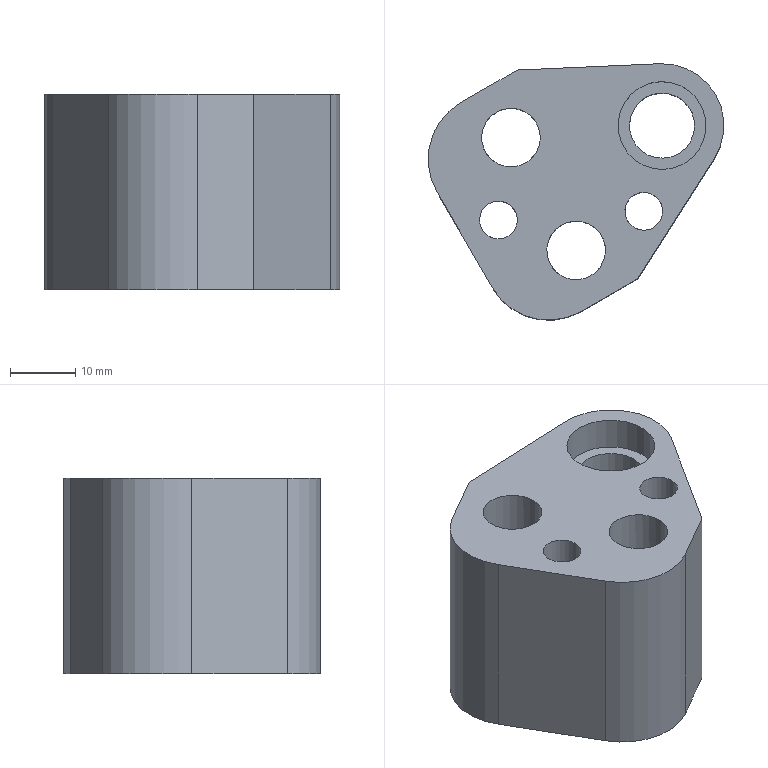Part | NX | features solid 2 | 1 solid | 25 faces | box 45.401 x 39.361 x 30 mm | volume 27576 mm3 | cylinder 13 | plane 12 | commonest cylinder face diameters 5.8 x2 8 x2 9 x2 14 x2 20 x2 10 x1
STEP:
#1=CARTESIAN_POINT('',(511.856,-185.624,74.));
#2=VERTEX_POINT('',#1);
#3=CARTESIAN_POINT('',(523.615,-167.196,74.));
#4=VERTEX_POINT('',#3);
#5=CARTESIAN_POINT('',(522.614,-168.764,74.));
#6=DIRECTION('',(0.5379,0.843,0.));
#7=VECTOR('',#6,1000.);
#8=LINE('',#5,#7);
#9=EDGE_CURVE('',#2,#4,#8,.T.);
#10=ORIENTED_EDGE('',*,*,#9,.T.);
#11=CARTESIAN_POINT('',(515.194,-152.611,74.));
#12=VERTEX_POINT('',#11);
#13=CARTESIAN_POINT('',(515.596,-162.103,74.));
#14=DIRECTION('',(0.,0.,-1.));
#15=DIRECTION('',(-0.5,0.866,0.));
#16=AXIS2_PLACEMENT_3D('',#13,#14,#15);
#17=CIRCLE('',#16,9.5);
#18=EDGE_CURVE('',#12,#4,#17,.T.);
#19=ORIENTED_EDGE('',*,*,#18,.F.);
#20=CARTESIAN_POINT('',(493.356,-153.581,74.));
#21=VERTEX_POINT('',#20);
#22=CARTESIAN_POINT('',(513.336,-152.694,74.));
#23=DIRECTION('',(-0.999,-0.04437,0.));
#24=VECTOR('',#23,1000.);
#25=LINE('',#22,#24);
#26=EDGE_CURVE('',#12,#21,#25,.T.);
#27=ORIENTED_EDGE('',*,*,#26,.T.);
#28=CARTESIAN_POINT('',(484.695,-158.581,74.));
#29=VERTEX_POINT('',#28);
#30=CARTESIAN_POINT('',(501.747,-148.736,74.));
#31=DIRECTION('',(0.866,0.5,0.));
#32=VECTOR('',#31,1000.);
#33=LINE('',#30,#32);
#34=EDGE_CURVE('',#29,#21,#33,.T.);
#35=ORIENTED_EDGE('',*,*,#34,.F.);
#36=CARTESIAN_POINT('',(481.035,-172.241,74.));
#37=VERTEX_POINT('',#36);
#38=CARTESIAN_POINT('',(489.695,-167.241,74.));
#39=DIRECTION('',(0.,0.,1.));
#40=DIRECTION('',(-0.5,-0.866,0.));
#41=AXIS2_PLACEMENT_3D('',#38,#39,#40);
#42=CIRCLE('',#41,10.);
#43=EDGE_CURVE('',#29,#37,#42,.T.);
#44=ORIENTED_EDGE('',*,*,#43,.T.);
#45=CARTESIAN_POINT('',(489.535,-186.964,74.));
#46=VERTEX_POINT('',#45);
#47=CARTESIAN_POINT('',(485.285,-179.603,74.));
#48=DIRECTION('',(-0.5,0.866,0.));
#49=VECTOR('',#48,1000.);
#50=LINE('',#47,#49);
#51=EDGE_CURVE('',#46,#37,#50,.T.);
#52=ORIENTED_EDGE('',*,*,#51,.F.);
#53=CARTESIAN_POINT('',(503.195,-190.624,74.));
#54=VERTEX_POINT('',#53);
#55=CARTESIAN_POINT('',(498.195,-181.964,74.));
#56=DIRECTION('',(0.,0.,1.));
#57=DIRECTION('',(-0.5,-0.866,0.));
#58=AXIS2_PLACEMENT_3D('',#55,#56,#57);
#59=CIRCLE('',#58,10.);
#60=EDGE_CURVE('',#46,#54,#59,.T.);
#61=ORIENTED_EDGE('',*,*,#60,.T.);
#62=CARTESIAN_POINT('',(520.247,-180.779,74.));
#63=DIRECTION('',(-0.866,-0.5,0.));
#64=VECTOR('',#63,1000.);
#65=LINE('',#62,#64);
#66=EDGE_CURVE('',#2,#54,#65,.T.);
#67=ORIENTED_EDGE('',*,*,#66,.F.);
#68=EDGE_LOOP('',(#10,#19,#27,#35,#44,#52,#61,#67));
#69=FACE_BOUND('',#68,.T.);
#70=CARTESIAN_POINT('',(489.031,-174.091,74.));
#71=VERTEX_POINT('',#70);
#72=CARTESIAN_POINT('',(490.481,-176.603,74.));
#73=DIRECTION('',(0.,0.,-1.));
#74=DIRECTION('',(-0.5,0.866,0.));
#75=AXIS2_PLACEMENT_3D('',#72,#73,#74);
#76=CIRCLE('',#75,2.9);
#77=EDGE_CURVE('',#71,#71,#76,.T.);
#78=ORIENTED_EDGE('',*,*,#77,.T.);
#79=EDGE_LOOP('',(#78));
#80=FACE_BOUND('',#79,.T.);
#81=CARTESIAN_POINT('',(511.352,-172.751,74.));
#82=VERTEX_POINT('',#81);
#83=CARTESIAN_POINT('',(512.802,-175.263,74.));
#84=DIRECTION('',(0.,0.,-1.));
#85=DIRECTION('',(-0.5,0.866,0.));
#86=AXIS2_PLACEMENT_3D('',#83,#84,#85);
#87=CIRCLE('',#86,2.9);
#88=EDGE_CURVE('',#82,#82,#87,.T.);
#89=ORIENTED_EDGE('',*,*,#88,.T.);
#90=EDGE_LOOP('',(#89));
#91=FACE_BOUND('',#90,.T.);
#92=CARTESIAN_POINT('',(500.159,-177.366,74.));
#93=VERTEX_POINT('',#92);
#94=CARTESIAN_POINT('',(502.409,-181.263,74.));
#95=DIRECTION('',(0.,0.,-1.));
#96=DIRECTION('',(-0.5,0.866,0.));
#97=AXIS2_PLACEMENT_3D('',#94,#95,#96);
#98=CIRCLE('',#97,4.5);
#99=EDGE_CURVE('',#93,#93,#98,.T.);
#100=ORIENTED_EDGE('',*,*,#99,.T.);
#101=EDGE_LOOP('',(#100));
#102=FACE_BOUND('',#101,.T.);
#103=CARTESIAN_POINT('',(490.159,-160.045,74.));
#104=VERTEX_POINT('',#103);
#105=CARTESIAN_POINT('',(492.409,-163.942,74.));
#106=DIRECTION('',(0.,0.,-1.));
#107=DIRECTION('',(-0.5,0.866,0.));
#108=AXIS2_PLACEMENT_3D('',#105,#106,#107);
#109=CIRCLE('',#108,4.5);
#110=EDGE_CURVE('',#104,#104,#109,.T.);
#111=ORIENTED_EDGE('',*,*,#110,.T.);
#112=EDGE_LOOP('',(#111));
#113=FACE_BOUND('',#112,.T.);
#114=CARTESIAN_POINT('',(512.221,-156.257,74.));
#115=VERTEX_POINT('',#114);
#116=CARTESIAN_POINT('',(515.596,-162.103,74.));
#117=DIRECTION('',(0.,0.,-1.));
#118=DIRECTION('',(-0.5,0.866,0.));
#119=AXIS2_PLACEMENT_3D('',#116,#117,#118);
#120=CIRCLE('',#119,6.75);
#121=EDGE_CURVE('',#115,#115,#120,.T.);
#122=ORIENTED_EDGE('',*,*,#121,.T.);
#123=EDGE_LOOP('',(#122));
#124=FACE_BOUND('',#123,.T.);
#125=CARTESIAN_POINT('',(510.997,-164.758,74.));
#126=DIRECTION('',(0.,0.,1.));
#127=DIRECTION('',(0.5,-0.866,0.));
#128=AXIS2_PLACEMENT_3D('',#125,#126,#127);
#129=PLANE('',#128);
#130=ADVANCED_FACE('',(#69,#80,#91,#102,#113,#124),#129,.T.);
#131=CARTESIAN_POINT('',(493.356,-153.581,44.));
#132=VERTEX_POINT('',#131);
#133=CARTESIAN_POINT('',(493.356,-153.581,44.));
#134=DIRECTION('',(0.,0.,1.));
#135=VECTOR('',#134,1000.);
#136=LINE('',#133,#135);
#137=EDGE_CURVE('',#132,#21,#136,.T.);
#138=ORIENTED_EDGE('',*,*,#137,.F.);
#139=CARTESIAN_POINT('',(484.695,-158.581,44.));
#140=VERTEX_POINT('',#139);
#141=CARTESIAN_POINT('',(501.747,-148.736,44.));
#142=DIRECTION('',(-0.866,-0.5,0.));
#143=VECTOR('',#142,1000.);
#144=LINE('',#141,#143);
#145=EDGE_CURVE('',#132,#140,#144,.T.);
#146=ORIENTED_EDGE('',*,*,#145,.T.);
#147=CARTESIAN_POINT('',(484.695,-158.581,44.));
#148=DIRECTION('',(0.,0.,1.));
#149=VECTOR('',#148,1000.);
#150=LINE('',#147,#149);
#151=EDGE_CURVE('',#140,#29,#150,.T.);
#152=ORIENTED_EDGE('',*,*,#151,.T.);
#153=ORIENTED_EDGE('',*,*,#34,.T.);
#154=EDGE_LOOP('',(#138,#146,#152,#153));
#155=FACE_BOUND('',#154,.T.);
#156=CARTESIAN_POINT('',(501.747,-148.736,44.));
#157=DIRECTION('',(-0.5,0.866,0.));
#158=DIRECTION('',(0.,0.,1.));
#159=AXIS2_PLACEMENT_3D('',#156,#157,#158);
#160=PLANE('',#159);
#161=ADVANCED_FACE('',(#155),#160,.T.);
#162=CARTESIAN_POINT('',(523.615,-167.196,44.));
#163=VERTEX_POINT('',#162);
#164=CARTESIAN_POINT('',(511.856,-185.624,44.));
#165=VERTEX_POINT('',#164);
#166=CARTESIAN_POINT('',(522.614,-168.764,44.));
#167=DIRECTION('',(-0.5379,-0.843,0.));
#168=VECTOR('',#167,1000.);
#169=LINE('',#166,#168);
#170=EDGE_CURVE('',#163,#165,#169,.T.);
#171=ORIENTED_EDGE('',*,*,#170,.T.);
#172=CARTESIAN_POINT('',(503.195,-190.624,44.));
#173=VERTEX_POINT('',#172);
#174=CARTESIAN_POINT('',(520.247,-180.779,44.));
#175=DIRECTION('',(0.866,0.5,0.));
#176=VECTOR('',#175,1000.);
#177=LINE('',#174,#176);
#178=EDGE_CURVE('',#173,#165,#177,.T.);
#179=ORIENTED_EDGE('',*,*,#178,.F.);
#180=CARTESIAN_POINT('',(489.535,-186.964,44.));
#181=VERTEX_POINT('',#180);
#182=CARTESIAN_POINT('',(498.195,-181.964,44.));
#183=DIRECTION('',(0.,0.,-1.));
#184=DIRECTION('',(0.5,0.866,0.));
#185=AXIS2_PLACEMENT_3D('',#182,#183,#184);
#186=CIRCLE('',#185,10.);
#187=EDGE_CURVE('',#173,#181,#186,.T.);
#188=ORIENTED_EDGE('',*,*,#187,.T.);
#189=CARTESIAN_POINT('',(481.035,-172.241,44.));
#190=VERTEX_POINT('',#189);
#191=CARTESIAN_POINT('',(485.285,-179.603,44.));
#192=DIRECTION('',(0.5,-0.866,0.));
#193=VECTOR('',#192,1000.);
#194=LINE('',#191,#193);
#195=EDGE_CURVE('',#190,#181,#194,.T.);
#196=ORIENTED_EDGE('',*,*,#195,.F.);
#197=CARTESIAN_POINT('',(489.695,-167.241,44.));
#198=DIRECTION('',(0.,0.,-1.));
#199=DIRECTION('',(0.5,0.866,0.));
#200=AXIS2_PLACEMENT_3D('',#197,#198,#199);
#201=CIRCLE('',#200,10.);
#202=EDGE_CURVE('',#190,#140,#201,.T.);
#203=ORIENTED_EDGE('',*,*,#202,.T.);
#204=ORIENTED_EDGE('',*,*,#145,.F.);
#205=CARTESIAN_POINT('',(515.194,-152.611,44.));
#206=VERTEX_POINT('',#205);
#207=CARTESIAN_POINT('',(513.336,-152.694,44.));
#208=DIRECTION('',(0.999,0.04437,0.));
#209=VECTOR('',#208,1000.);
#210=LINE('',#207,#209);
#211=EDGE_CURVE('',#132,#206,#210,.T.);
#212=ORIENTED_EDGE('',*,*,#211,.T.);
#213=CARTESIAN_POINT('',(515.596,-162.103,44.));
#214=DIRECTION('',(0.,0.,1.));
#215=DIRECTION('',(0.5,-0.866,0.));
#216=AXIS2_PLACEMENT_3D('',#213,#214,#215);
#217=CIRCLE('',#216,9.5);
#218=EDGE_CURVE('',#163,#206,#217,.T.);
#219=ORIENTED_EDGE('',*,*,#218,.F.);
#220=EDGE_LOOP('',(#171,#179,#188,#196,#203,#204,#212,#219));
#221=FACE_BOUND('',#220,.T.);
#222=CARTESIAN_POINT('',(492.481,-180.067,44.));
#223=VERTEX_POINT('',#222);
#224=CARTESIAN_POINT('',(490.481,-176.603,44.));
#225=DIRECTION('',(0.,0.,1.));
#226=DIRECTION('',(0.5,-0.866,0.));
#227=AXIS2_PLACEMENT_3D('',#224,#225,#226);
#228=CIRCLE('',#227,4.);
#229=EDGE_CURVE('',#223,#223,#228,.T.);
#230=ORIENTED_EDGE('',*,*,#229,.T.);
#231=EDGE_LOOP('',(#230));
#232=FACE_BOUND('',#231,.T.);
#233=CARTESIAN_POINT('',(514.802,-178.727,44.));
#234=VERTEX_POINT('',#233);
#235=CARTESIAN_POINT('',(512.802,-175.263,44.));
#236=DIRECTION('',(0.,0.,1.));
#237=DIRECTION('',(0.5,-0.866,0.));
#238=AXIS2_PLACEMENT_3D('',#235,#236,#237);
#239=CIRCLE('',#238,4.);
#240=EDGE_CURVE('',#234,#234,#239,.T.);
#241=ORIENTED_EDGE('',*,*,#240,.T.);
#242=EDGE_LOOP('',(#241));
#243=FACE_BOUND('',#242,.T.);
#244=CARTESIAN_POINT('',(505.909,-187.325,44.));
#245=VERTEX_POINT('',#244);
#246=CARTESIAN_POINT('',(502.409,-181.263,44.));
#247=DIRECTION('',(0.,0.,1.));
#248=DIRECTION('',(0.5,-0.866,0.));
#249=AXIS2_PLACEMENT_3D('',#246,#247,#248);
#250=CIRCLE('',#249,7.);
#251=EDGE_CURVE('',#245,#245,#250,.T.);
#252=ORIENTED_EDGE('',*,*,#251,.T.);
#253=EDGE_LOOP('',(#252));
#254=FACE_BOUND('',#253,.T.);
#255=CARTESIAN_POINT('',(495.909,-170.004,44.));
#256=VERTEX_POINT('',#255);
#257=CARTESIAN_POINT('',(492.409,-163.942,44.));
#258=DIRECTION('',(0.,0.,1.));
#259=DIRECTION('',(0.5,-0.866,0.));
#260=AXIS2_PLACEMENT_3D('',#257,#258,#259);
#261=CIRCLE('',#260,7.);
#262=EDGE_CURVE('',#256,#256,#261,.T.);
#263=ORIENTED_EDGE('',*,*,#262,.T.);
#264=EDGE_LOOP('',(#263));
#265=FACE_BOUND('',#264,.T.);
#266=CARTESIAN_POINT('',(518.096,-166.433,44.));
#267=VERTEX_POINT('',#266);
#268=CARTESIAN_POINT('',(515.596,-162.103,44.));
#269=DIRECTION('',(0.,0.,1.));
#270=DIRECTION('',(0.5,-0.866,0.));
#271=AXIS2_PLACEMENT_3D('',#268,#269,#270);
#272=CIRCLE('',#271,5.);
#273=EDGE_CURVE('',#267,#267,#272,.T.);
#274=ORIENTED_EDGE('',*,*,#273,.T.);
#275=EDGE_LOOP('',(#274));
#276=FACE_BOUND('',#275,.T.);
#277=CARTESIAN_POINT('',(510.997,-164.758,44.));
#278=DIRECTION('',(0.,0.,-1.));
#279=DIRECTION('',(-0.5,0.866,0.));
#280=AXIS2_PLACEMENT_3D('',#277,#278,#279);
#281=PLANE('',#280);
#282=ADVANCED_FACE('',(#221,#232,#243,#254,#265,#276),#281,.T.);
#283=CARTESIAN_POINT('',(511.856,-185.624,44.));
#284=DIRECTION('',(0.,0.,1.));
#285=VECTOR('',#284,1000.);
#286=LINE('',#283,#285);
#287=EDGE_CURVE('',#165,#2,#286,.T.);
#288=ORIENTED_EDGE('',*,*,#287,.T.);
#289=ORIENTED_EDGE('',*,*,#66,.T.);
#290=CARTESIAN_POINT('',(503.195,-190.624,44.));
#291=DIRECTION('',(0.,0.,1.));
#292=VECTOR('',#291,1000.);
#293=LINE('',#290,#292);
#294=EDGE_CURVE('',#54,#173,#293,.F.);
#295=ORIENTED_EDGE('',*,*,#294,.T.);
#296=ORIENTED_EDGE('',*,*,#178,.T.);
#297=EDGE_LOOP('',(#288,#289,#295,#296));
#298=FACE_BOUND('',#297,.T.);
#299=CARTESIAN_POINT('',(520.247,-180.779,44.));
#300=DIRECTION('',(0.5,-0.866,0.));
#301=DIRECTION('',(0.,0.,-1.));
#302=AXIS2_PLACEMENT_3D('',#299,#300,#301);
#303=PLANE('',#302);
#304=ADVANCED_FACE('',(#298),#303,.T.);
#305=CARTESIAN_POINT('',(523.615,-167.196,74.));
#306=DIRECTION('',(0.,0.,-1.));
#307=VECTOR('',#306,1000.);
#308=LINE('',#305,#307);
#309=EDGE_CURVE('',#163,#4,#308,.F.);
#310=ORIENTED_EDGE('',*,*,#309,.F.);
#311=ORIENTED_EDGE('',*,*,#218,.T.);
#312=CARTESIAN_POINT('',(515.194,-152.611,74.));
#313=DIRECTION('',(0.,0.,-1.));
#314=VECTOR('',#313,1000.);
#315=LINE('',#312,#314);
#316=EDGE_CURVE('',#12,#206,#315,.T.);
#317=ORIENTED_EDGE('',*,*,#316,.F.);
#318=ORIENTED_EDGE('',*,*,#18,.T.);
#319=EDGE_LOOP('',(#310,#311,#317,#318));
#320=FACE_BOUND('',#319,.T.);
#321=CARTESIAN_POINT('',(515.596,-162.103,74.));
#322=DIRECTION('',(0.,0.,-1.));
#323=DIRECTION('',(-0.5,0.866,0.));
#324=AXIS2_PLACEMENT_3D('',#321,#322,#323);
#325=CYLINDRICAL_SURFACE('',#324,9.5);
#326=ADVANCED_FACE('',(#320),#325,.T.);
#327=ORIENTED_EDGE('',*,*,#195,.T.);
#328=CARTESIAN_POINT('',(489.535,-186.964,44.));
#329=DIRECTION('',(0.,0.,1.));
#330=VECTOR('',#329,1000.);
#331=LINE('',#328,#330);
#332=EDGE_CURVE('',#181,#46,#331,.T.);
#333=ORIENTED_EDGE('',*,*,#332,.T.);
#334=ORIENTED_EDGE('',*,*,#51,.T.);
#335=CARTESIAN_POINT('',(481.035,-172.241,44.));
#336=DIRECTION('',(0.,0.,1.));
#337=VECTOR('',#336,1000.);
#338=LINE('',#335,#337);
#339=EDGE_CURVE('',#37,#190,#338,.F.);
#340=ORIENTED_EDGE('',*,*,#339,.T.);
#341=EDGE_LOOP('',(#327,#333,#334,#340));
#342=FACE_BOUND('',#341,.T.);
#343=CARTESIAN_POINT('',(485.285,-179.603,44.));
#344=DIRECTION('',(-0.866,-0.5,0.));
#345=DIRECTION('',(0.,0.,-1.));
#346=AXIS2_PLACEMENT_3D('',#343,#344,#345);
#347=PLANE('',#346);
#348=ADVANCED_FACE('',(#342),#347,.T.);
#349=CARTESIAN_POINT('',(513.096,-157.772,69.));
#350=VERTEX_POINT('',#349);
#351=CARTESIAN_POINT('',(515.596,-162.103,69.));
#352=DIRECTION('',(0.,0.,-1.));
#353=DIRECTION('',(-0.5,0.866,0.));
#354=AXIS2_PLACEMENT_3D('',#351,#352,#353);
#355=CIRCLE('',#354,5.);
#356=EDGE_CURVE('',#350,#350,#355,.T.);
#357=ORIENTED_EDGE('',*,*,#356,.T.);
#358=EDGE_LOOP('',(#357));
#359=FACE_BOUND('',#358,.T.);
#360=CARTESIAN_POINT('',(518.971,-167.948,69.));
#361=VERTEX_POINT('',#360);
#362=CARTESIAN_POINT('',(515.596,-162.103,69.));
#363=DIRECTION('',(0.,0.,1.));
#364=DIRECTION('',(0.5,-0.866,0.));
#365=AXIS2_PLACEMENT_3D('',#362,#363,#364);
#366=CIRCLE('',#365,6.75);
#367=EDGE_CURVE('',#361,#361,#366,.T.);
#368=ORIENTED_EDGE('',*,*,#367,.T.);
#369=EDGE_LOOP('',(#368));
#370=FACE_BOUND('',#369,.T.);
#371=CARTESIAN_POINT('',(515.596,-162.103,69.));
#372=DIRECTION('',(0.,0.,-1.));
#373=DIRECTION('',(-0.5,0.866,0.));
#374=AXIS2_PLACEMENT_3D('',#371,#372,#373);
#375=PLANE('',#374);
#376=ADVANCED_FACE('',(#359,#370),#375,.F.);
#377=ORIENTED_EDGE('',*,*,#367,.F.);
#378=EDGE_LOOP('',(#377));
#379=FACE_BOUND('',#378,.T.);
#380=ORIENTED_EDGE('',*,*,#121,.F.);
#381=EDGE_LOOP('',(#380));
#382=FACE_BOUND('',#381,.T.);
#383=CARTESIAN_POINT('',(515.596,-162.103,74.));
#384=DIRECTION('',(0.,0.,-1.));
#385=DIRECTION('',(-0.5,0.866,0.));
#386=AXIS2_PLACEMENT_3D('',#383,#384,#385);
#387=CYLINDRICAL_SURFACE('',#386,6.75);
#388=ADVANCED_FACE('',(#379,#382),#387,.F.);
#389=ORIENTED_EDGE('',*,*,#273,.F.);
#390=EDGE_LOOP('',(#389));
#391=FACE_BOUND('',#390,.T.);
#392=ORIENTED_EDGE('',*,*,#356,.F.);
#393=EDGE_LOOP('',(#392));
#394=FACE_BOUND('',#393,.T.);
#395=CARTESIAN_POINT('',(515.596,-162.103,69.));
#396=DIRECTION('',(0.,0.,-1.));
#397=DIRECTION('',(-0.5,0.866,0.));
#398=AXIS2_PLACEMENT_3D('',#395,#396,#397);
#399=CYLINDRICAL_SURFACE('',#398,5.);
#400=ADVANCED_FACE('',(#391,#394),#399,.F.);
#401=CARTESIAN_POINT('',(490.159,-167.839,54.));
#402=VERTEX_POINT('',#401);
#403=CARTESIAN_POINT('',(492.409,-163.942,54.));
#404=DIRECTION('',(0.,0.,1.));
#405=DIRECTION('',(-0.5,-0.866,0.));
#406=AXIS2_PLACEMENT_3D('',#403,#404,#405);
#407=CIRCLE('',#406,4.5);
#408=EDGE_CURVE('',#402,#402,#407,.F.);
#409=ORIENTED_EDGE('',*,*,#408,.T.);
#410=EDGE_LOOP('',(#409));
#411=FACE_BOUND('',#410,.T.);
#412=ORIENTED_EDGE('',*,*,#110,.F.);
#413=EDGE_LOOP('',(#412));
#414=FACE_BOUND('',#413,.T.);
#415=CARTESIAN_POINT('',(492.409,-163.942,74.));
#416=DIRECTION('',(0.,0.,-1.));
#417=DIRECTION('',(-0.5,0.866,0.));
#418=AXIS2_PLACEMENT_3D('',#415,#416,#417);
#419=CYLINDRICAL_SURFACE('',#418,4.5);
#420=ADVANCED_FACE('',(#411,#414),#419,.F.);
#421=CARTESIAN_POINT('',(488.909,-157.88,54.));
#422=VERTEX_POINT('',#421);
#423=CARTESIAN_POINT('',(492.409,-163.942,54.));
#424=DIRECTION('',(0.,0.,-1.));
#425=DIRECTION('',(-0.5,0.866,0.));
#426=AXIS2_PLACEMENT_3D('',#423,#424,#425);
#427=CIRCLE('',#426,7.);
#428=EDGE_CURVE('',#422,#422,#427,.T.);
#429=ORIENTED_EDGE('',*,*,#428,.T.);
#430=EDGE_LOOP('',(#429));
#431=FACE_BOUND('',#430,.T.);
#432=ORIENTED_EDGE('',*,*,#408,.F.);
#433=EDGE_LOOP('',(#432));
#434=FACE_BOUND('',#433,.T.);
#435=CARTESIAN_POINT('',(492.409,-163.942,54.));
#436=DIRECTION('',(0.,0.,1.));
#437=DIRECTION('',(0.5,-0.866,0.));
#438=AXIS2_PLACEMENT_3D('',#435,#436,#437);
#439=PLANE('',#438);
#440=ADVANCED_FACE('',(#431,#434),#439,.F.);
#441=ORIENTED_EDGE('',*,*,#262,.F.);
#442=EDGE_LOOP('',(#441));
#443=FACE_BOUND('',#442,.T.);
#444=ORIENTED_EDGE('',*,*,#428,.F.);
#445=EDGE_LOOP('',(#444));
#446=FACE_BOUND('',#445,.T.);
#447=CARTESIAN_POINT('',(492.409,-163.942,54.));
#448=DIRECTION('',(0.,0.,-1.));
#449=DIRECTION('',(-0.5,0.866,0.));
#450=AXIS2_PLACEMENT_3D('',#447,#448,#449);
#451=CYLINDRICAL_SURFACE('',#450,7.);
#452=ADVANCED_FACE('',(#443,#446),#451,.F.);
#453=CARTESIAN_POINT('',(500.159,-185.16,54.));
#454=VERTEX_POINT('',#453);
#455=CARTESIAN_POINT('',(502.409,-181.263,54.));
#456=DIRECTION('',(0.,0.,1.));
#457=DIRECTION('',(-0.5,-0.866,0.));
#458=AXIS2_PLACEMENT_3D('',#455,#456,#457);
#459=CIRCLE('',#458,4.5);
#460=EDGE_CURVE('',#454,#454,#459,.F.);
#461=ORIENTED_EDGE('',*,*,#460,.T.);
#462=EDGE_LOOP('',(#461));
#463=FACE_BOUND('',#462,.T.);
#464=ORIENTED_EDGE('',*,*,#99,.F.);
#465=EDGE_LOOP('',(#464));
#466=FACE_BOUND('',#465,.T.);
#467=CARTESIAN_POINT('',(502.409,-181.263,74.));
#468=DIRECTION('',(0.,0.,-1.));
#469=DIRECTION('',(-0.5,0.866,0.));
#470=AXIS2_PLACEMENT_3D('',#467,#468,#469);
#471=CYLINDRICAL_SURFACE('',#470,4.5);
#472=ADVANCED_FACE('',(#463,#466),#471,.F.);
#473=CARTESIAN_POINT('',(498.909,-175.201,54.));
#474=VERTEX_POINT('',#473);
#475=CARTESIAN_POINT('',(502.409,-181.263,54.));
#476=DIRECTION('',(0.,0.,-1.));
#477=DIRECTION('',(-0.5,0.866,0.));
#478=AXIS2_PLACEMENT_3D('',#475,#476,#477);
#479=CIRCLE('',#478,7.);
#480=EDGE_CURVE('',#474,#474,#479,.T.);
#481=ORIENTED_EDGE('',*,*,#480,.T.);
#482=EDGE_LOOP('',(#481));
#483=FACE_BOUND('',#482,.T.);
#484=ORIENTED_EDGE('',*,*,#460,.F.);
#485=EDGE_LOOP('',(#484));
#486=FACE_BOUND('',#485,.T.);
#487=CARTESIAN_POINT('',(502.409,-181.263,54.));
#488=DIRECTION('',(0.,0.,1.));
#489=DIRECTION('',(0.5,-0.866,0.));
#490=AXIS2_PLACEMENT_3D('',#487,#488,#489);
#491=PLANE('',#490);
#492=ADVANCED_FACE('',(#483,#486),#491,.F.);
#493=ORIENTED_EDGE('',*,*,#251,.F.);
#494=EDGE_LOOP('',(#493));
#495=FACE_BOUND('',#494,.T.);
#496=ORIENTED_EDGE('',*,*,#480,.F.);
#497=EDGE_LOOP('',(#496));
#498=FACE_BOUND('',#497,.T.);
#499=CARTESIAN_POINT('',(502.409,-181.263,54.));
#500=DIRECTION('',(0.,0.,-1.));
#501=DIRECTION('',(-0.5,0.866,0.));
#502=AXIS2_PLACEMENT_3D('',#499,#500,#501);
#503=CYLINDRICAL_SURFACE('',#502,7.);
#504=ADVANCED_FACE('',(#495,#498),#503,.F.);
#505=CARTESIAN_POINT('',(511.352,-177.774,64.));
#506=VERTEX_POINT('',#505);
#507=CARTESIAN_POINT('',(512.802,-175.263,64.));
#508=DIRECTION('',(0.,0.,1.));
#509=DIRECTION('',(-0.5,-0.866,0.));
#510=AXIS2_PLACEMENT_3D('',#507,#508,#509);
#511=CIRCLE('',#510,2.9);
#512=EDGE_CURVE('',#506,#506,#511,.F.);
#513=ORIENTED_EDGE('',*,*,#512,.T.);
#514=EDGE_LOOP('',(#513));
#515=FACE_BOUND('',#514,.T.);
#516=ORIENTED_EDGE('',*,*,#88,.F.);
#517=EDGE_LOOP('',(#516));
#518=FACE_BOUND('',#517,.T.);
#519=CARTESIAN_POINT('',(512.802,-175.263,74.));
#520=DIRECTION('',(0.,0.,-1.));
#521=DIRECTION('',(-0.5,0.866,0.));
#522=AXIS2_PLACEMENT_3D('',#519,#520,#521);
#523=CYLINDRICAL_SURFACE('',#522,2.9);
#524=ADVANCED_FACE('',(#515,#518),#523,.F.);
#525=CARTESIAN_POINT('',(510.802,-171.799,64.));
#526=VERTEX_POINT('',#525);
#527=CARTESIAN_POINT('',(512.802,-175.263,64.));
#528=DIRECTION('',(0.,0.,-1.));
#529=DIRECTION('',(-0.5,0.866,0.));
#530=AXIS2_PLACEMENT_3D('',#527,#528,#529);
#531=CIRCLE('',#530,4.);
#532=EDGE_CURVE('',#526,#526,#531,.T.);
#533=ORIENTED_EDGE('',*,*,#532,.T.);
#534=EDGE_LOOP('',(#533));
#535=FACE_BOUND('',#534,.T.);
#536=ORIENTED_EDGE('',*,*,#512,.F.);
#537=EDGE_LOOP('',(#536));
#538=FACE_BOUND('',#537,.T.);
#539=CARTESIAN_POINT('',(512.802,-175.263,64.));
#540=DIRECTION('',(0.,0.,1.));
#541=DIRECTION('',(0.5,-0.866,0.));
#542=AXIS2_PLACEMENT_3D('',#539,#540,#541);
#543=PLANE('',#542);
#544=ADVANCED_FACE('',(#535,#538),#543,.F.);
#545=ORIENTED_EDGE('',*,*,#240,.F.);
#546=EDGE_LOOP('',(#545));
#547=FACE_BOUND('',#546,.T.);
#548=ORIENTED_EDGE('',*,*,#532,.F.);
#549=EDGE_LOOP('',(#548));
#550=FACE_BOUND('',#549,.T.);
#551=CARTESIAN_POINT('',(512.802,-175.263,64.));
#552=DIRECTION('',(0.,0.,-1.));
#553=DIRECTION('',(-0.5,0.866,0.));
#554=AXIS2_PLACEMENT_3D('',#551,#552,#553);
#555=CYLINDRICAL_SURFACE('',#554,4.);
#556=ADVANCED_FACE('',(#547,#550),#555,.F.);
#557=CARTESIAN_POINT('',(489.031,-179.114,64.));
#558=VERTEX_POINT('',#557);
#559=CARTESIAN_POINT('',(490.481,-176.603,64.));
#560=DIRECTION('',(0.,0.,1.));
#561=DIRECTION('',(-0.5,-0.866,0.));
#562=AXIS2_PLACEMENT_3D('',#559,#560,#561);
#563=CIRCLE('',#562,2.9);
#564=EDGE_CURVE('',#558,#558,#563,.F.);
#565=ORIENTED_EDGE('',*,*,#564,.T.);
#566=EDGE_LOOP('',(#565));
#567=FACE_BOUND('',#566,.T.);
#568=ORIENTED_EDGE('',*,*,#77,.F.);
#569=EDGE_LOOP('',(#568));
#570=FACE_BOUND('',#569,.T.);
#571=CARTESIAN_POINT('',(490.481,-176.603,74.));
#572=DIRECTION('',(0.,0.,-1.));
#573=DIRECTION('',(-0.5,0.866,0.));
#574=AXIS2_PLACEMENT_3D('',#571,#572,#573);
#575=CYLINDRICAL_SURFACE('',#574,2.9);
#576=ADVANCED_FACE('',(#567,#570),#575,.F.);
#577=CARTESIAN_POINT('',(488.481,-173.138,64.));
#578=VERTEX_POINT('',#577);
#579=CARTESIAN_POINT('',(490.481,-176.603,64.));
#580=DIRECTION('',(0.,0.,-1.));
#581=DIRECTION('',(-0.5,0.866,0.));
#582=AXIS2_PLACEMENT_3D('',#579,#580,#581);
#583=CIRCLE('',#582,4.);
#584=EDGE_CURVE('',#578,#578,#583,.T.);
#585=ORIENTED_EDGE('',*,*,#584,.T.);
#586=EDGE_LOOP('',(#585));
#587=FACE_BOUND('',#586,.T.);
#588=ORIENTED_EDGE('',*,*,#564,.F.);
#589=EDGE_LOOP('',(#588));
#590=FACE_BOUND('',#589,.T.);
#591=CARTESIAN_POINT('',(490.481,-176.603,64.));
#592=DIRECTION('',(0.,0.,1.));
#593=DIRECTION('',(0.5,-0.866,0.));
#594=AXIS2_PLACEMENT_3D('',#591,#592,#593);
#595=PLANE('',#594);
#596=ADVANCED_FACE('',(#587,#590),#595,.F.);
#597=ORIENTED_EDGE('',*,*,#229,.F.);
#598=EDGE_LOOP('',(#597));
#599=FACE_BOUND('',#598,.T.);
#600=ORIENTED_EDGE('',*,*,#584,.F.);
#601=EDGE_LOOP('',(#600));
#602=FACE_BOUND('',#601,.T.);
#603=CARTESIAN_POINT('',(490.481,-176.603,64.));
#604=DIRECTION('',(0.,0.,-1.));
#605=DIRECTION('',(-0.5,0.866,0.));
#606=AXIS2_PLACEMENT_3D('',#603,#604,#605);
#607=CYLINDRICAL_SURFACE('',#606,4.);
#608=ADVANCED_FACE('',(#599,#602),#607,.F.);
#609=ORIENTED_EDGE('',*,*,#187,.F.);
#610=ORIENTED_EDGE('',*,*,#294,.F.);
#611=ORIENTED_EDGE('',*,*,#60,.F.);
#612=ORIENTED_EDGE('',*,*,#332,.F.);
#613=EDGE_LOOP('',(#609,#610,#611,#612));
#614=FACE_BOUND('',#613,.T.);
#615=CARTESIAN_POINT('',(498.195,-181.964,44.));
#616=DIRECTION('',(0.,0.,1.));
#617=DIRECTION('',(-0.5,-0.866,0.));
#618=AXIS2_PLACEMENT_3D('',#615,#616,#617);
#619=CYLINDRICAL_SURFACE('',#618,10.);
#620=ADVANCED_FACE('',(#614),#619,.T.);
#621=ORIENTED_EDGE('',*,*,#202,.F.);
#622=ORIENTED_EDGE('',*,*,#339,.F.);
#623=ORIENTED_EDGE('',*,*,#43,.F.);
#624=ORIENTED_EDGE('',*,*,#151,.F.);
#625=EDGE_LOOP('',(#621,#622,#623,#624));
#626=FACE_BOUND('',#625,.T.);
#627=CARTESIAN_POINT('',(489.695,-167.241,44.));
#628=DIRECTION('',(0.,0.,1.));
#629=DIRECTION('',(-0.5,-0.866,0.));
#630=AXIS2_PLACEMENT_3D('',#627,#628,#629);
#631=CYLINDRICAL_SURFACE('',#630,10.);
#632=ADVANCED_FACE('',(#626),#631,.T.);
#633=ORIENTED_EDGE('',*,*,#316,.T.);
#634=ORIENTED_EDGE('',*,*,#211,.F.);
#635=ORIENTED_EDGE('',*,*,#137,.T.);
#636=ORIENTED_EDGE('',*,*,#26,.F.);
#637=EDGE_LOOP('',(#633,#634,#635,#636));
#638=FACE_BOUND('',#637,.T.);
#639=CARTESIAN_POINT('',(513.336,-152.694,44.));
#640=DIRECTION('',(0.04437,-0.999,0.));
#641=DIRECTION('',(0.,0.,-1.));
#642=AXIS2_PLACEMENT_3D('',#639,#640,#641);
#643=PLANE('',#642);
#644=ADVANCED_FACE('',(#638),#643,.F.);
#645=ORIENTED_EDGE('',*,*,#309,.T.);
#646=ORIENTED_EDGE('',*,*,#9,.F.);
#647=ORIENTED_EDGE('',*,*,#287,.F.);
#648=ORIENTED_EDGE('',*,*,#170,.F.);
#649=EDGE_LOOP('',(#645,#646,#647,#648));
#650=FACE_BOUND('',#649,.T.);
#651=CARTESIAN_POINT('',(522.614,-168.764,44.));
#652=DIRECTION('',(-0.843,0.5379,0.));
#653=DIRECTION('',(0.,0.,1.));
#654=AXIS2_PLACEMENT_3D('',#651,#652,#653);
#655=PLANE('',#654);
#656=ADVANCED_FACE('',(#650),#655,.F.);
#657=CLOSED_SHELL('',(#130,#161,#282,#304,#326,#348,#376,#388,#400,#420,#440,#452,#472,#492,#504,#524,#544,#556,#576,#596,#608,#620,#632,#644,#656));
#658=MANIFOLD_SOLID_BREP('',#657);
#659=(LENGTH_UNIT()NAMED_UNIT(*)SI_UNIT(.MILLI.,.METRE.));
#660=UNCERTAINTY_MEASURE_WITH_UNIT(LENGTH_MEASURE(0.00001),#659,'','');
#661=(NAMED_UNIT(*)PLANE_ANGLE_UNIT()SI_UNIT($,.RADIAN.));
#662=(NAMED_UNIT(*)SI_UNIT($,.STERADIAN.)SOLID_ANGLE_UNIT());
#663=(GEOMETRIC_REPRESENTATION_CONTEXT(3)GLOBAL_UNCERTAINTY_ASSIGNED_CONTEXT((#660))GLOBAL_UNIT_ASSIGNED_CONTEXT((#659,#661,#662))REPRESENTATION_CONTEXT('',''));
#664=ADVANCED_BREP_SHAPE_REPRESENTATION('',(#658),#663);